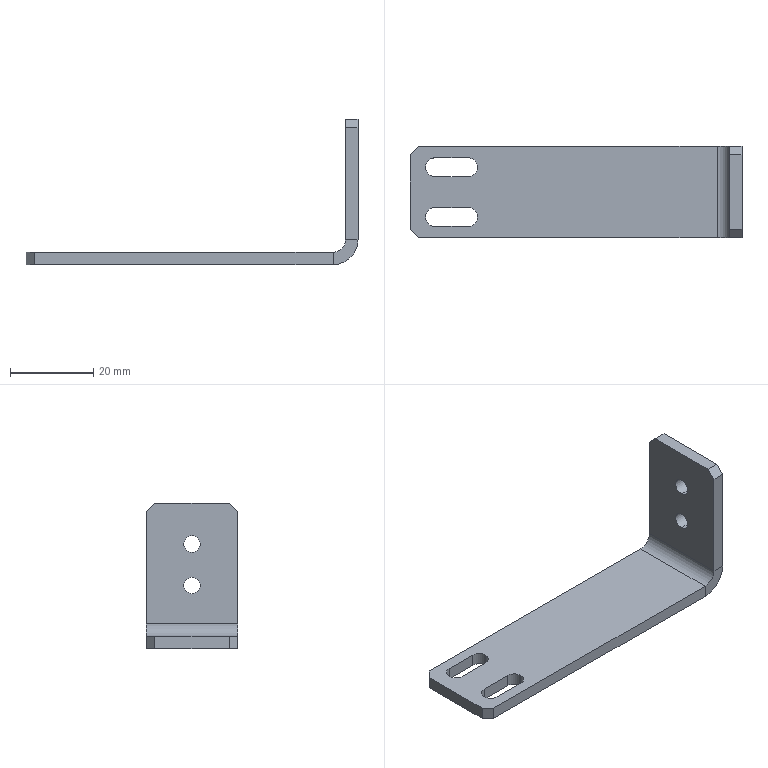Part | STEP file | ASND-0110-Body 1-11 | 1 solid | 32 faces | box 80 x 22 x 35 mm | volume 6854 mm3 | plane 20 | cylinder 12 | commonest cylinder face diameters 4.5 x6 4 x4 6 x1 12 x1